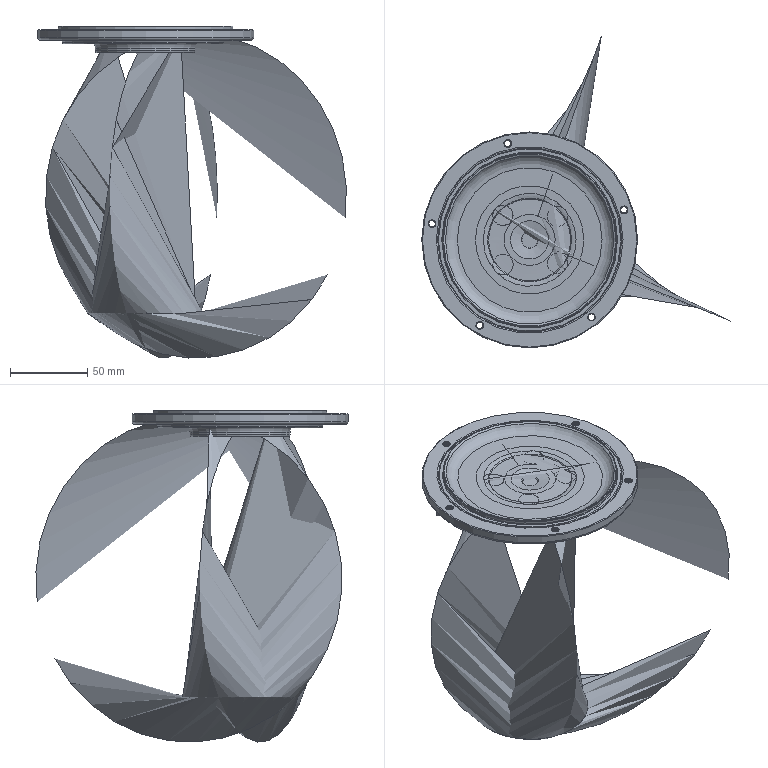CAM job | NX | 3-axis milling, drilling
Tools:
number,name,description,diameter,corner_radius,flute_length,length,flutes
1,D63,Milling Tool-5 Parameters,63.0,0.0,50.0,75.0,2
10,D10,Milling Tool-5 Parameters,10.0,0.0,50.0,75.0,2
11,D10JING,Milling Tool-5 Parameters,10.0,0.0,50.0,75.0,2
6,D6,Milling Tool-5 Parameters,6.0,0.0,50.0,75.0,2
5,D6R0.5,Milling Tool-5 Parameters,6.0,0.5,50.0,75.0,2
2,R0.5,Milling Tool-5 Parameters,1.0,0.5,50.0,75.0,2
7,D6A45,Milling Tool-5 Parameters,6.0,0.0,50.0,75.0,2
3,D3,Milling Tool-5 Parameters,3.0,0.0,50.0,75.0,2
14,4.2ZT,Drilling Tool,4.2,0.0,35.0,50.0,2
16,6.6ZT,Drilling Tool,6.6,0.0,35.0,50.0,2
8,R1.5,Milling Tool-5 Parameters,3.0,1.5,30.0,30.0,4
Operations:
program,operation,operation_type,tool,method,geometry_group,spindle_rpm,surface_speed,feed_per_tooth,feed_cut,feed_plunge,cut_length_mm,path_length_mm,cut_time_min,machine_time_min
1,FLOOR_WALL,VolumeBased25DMillingOperation,D63,METHOD,A,6500.0,1286.0,0.0962,1250.0,100.0,987.547,1041.547,0.79,0.7954
1,ADAPTIVE_MILLING,CavityMilling,D10,METHOD,A,9500.0,298.0,0.1579,3000.0,1000.0,12242.266,12331.08,4.083,4.092
1,CAVITY_MILL,CavityMilling,D10,METHOD,A,9500.0,298.0,0.1579,3000.0,1000.0,13987.132,15102.325,5.036,5.148
1,FLOOR_WALL_1,VolumeBased25DMillingOperation,D10JING,METHOD,A,9500.0,298.0,0.0658,1250.0,100.0,1641.55,1704.25,1.313,1.319
1,ZLEVEL_PROFILE_1,ZLevelMilling,D10JING,METHOD,A,9500.0,298.0,0.0658,1250.0,100.0,478.967,570.782,0.3832,0.3924
1,HOLE_MILLING,CylinderMilling,D6,METHOD,A,9500.0,179.0,0.1053,2000.0,100.0,162.988,239.015,0.0815,0.0891
1,FIXED_CONTOUR,SurfaceContour,D6R0.5,METHOD,A,9500.0,179.0,0.1842,3500.0,1000.0,90276.733,90348.728,25.801,25.808
1,ZLEVEL_PROFILE,ZLevelMilling,D6R0.5,METHOD,A,9500.0,179.0,0.1842,3500.0,1000.0,9728.054,9788.404,2.794,2.8
1,FIXED_CONTOUR_COPY,SurfaceContour,R0.5,METHOD,A,9500.0,179.0,0.1842,3500.0,1000.0,11634.403,11692.003,3.327,3.332
1,PLANAR_MILL,PlanarMilling,D6A45,METHOD,A,9500.0,179.0,0.0789,1500.0,100.0,452.006,516.706,0.3013,0.3078
2,FLOOR_WALL_COPY,VolumeBased25DMillingOperation,D63,METHOD,B,6500.0,1286.0,0.0962,1250.0,100.0,2830.641,3215.735,2.264,2.303
2,CAVITY_MILL_COPY,CavityMilling,D10,METHOD,B,9500.0,298.0,0.1579,3000.0,750.0,28269.25,29278.125,9.95,10.051
2,FLOOR_WALL_1_COPY,VolumeBased25DMillingOperation,D10JING,METHOD,B,9500.0,298.0,0.0658,1250.0,100.0,1599.832,1673.947,1.28,1.287
2,FLOOR_WALL_1_COPY_COPY,VolumeBased25DMillingOperation,D10JING,METHOD,B,9500.0,298.0,0.0658,1250.0,100.0,598.138,663.538,0.4785,0.4851
2,CAVITY_MILL_COPY_COPY,CavityMilling,D6,METHOD,B,9500.0,179.0,0.1053,2000.0,1000.0,1351.467,1851.156,0.7828,0.8328
2,CAVITY_MILL_COPY_COPY_COPY,CavityMilling,D3,METHOD,B,9500.0,89.0,0.0711,1350.0,1000.0,404.339,735.835,0.3226,0.3558
2,DRILLING,Operation,D6A45,METHOD,B,5000.0,94.0,0.025,250.0,0.0,28.0,433.346,0.112,0.1525
2,DRILLING_COPY,Operation,D6A45,METHOD,B,5000.0,94.0,0.025,250.0,0.0,22.4,218.986,0.0896,0.1093
2,DRILLING_COPY_1,Operation,4.2ZT,METHOD,B,2000.0,26.0,0.0625,250.0,0.0,61.309,499.964,0.2452,0.2891
2,DRILLING_COPY_COPY,Operation,6.6ZT,METHOD,B,2000.0,41.0,0.0625,250.0,0.0,59.931,294.049,0.2397,0.2631
2,PLANAR_MILL_COPY,PlanarMilling,D6A45,METHOD,B,9500.0,179.0,0.0789,1500.0,100.0,85.363,452.323,0.0569,0.0936
2,ZLEVEL_PROFILE_COPY,ZLevelMilling,D6R0.5,METHOD,B,9500.0,179.0,0.1842,3500.0,1000.0,3101.647,3173.346,0.9003,0.9074
2,FIXED_CONTOUR_COPY_1_COPY_COPY,SurfaceContour,D6R0.5,METHOD,B,9500.0,179.0,0.1842,3500.0,1000.0,70122.253,70181.666,20.038,20.044
2,ZLEVEL_PROFILE_COPY_1,ZLevelMilling,D6R0.5,METHOD,B,9500.0,179.0,0.1842,3500.0,1000.0,17246.31,17322.924,4.941,4.949
2,ZLEVEL_PROFILE_COPY_1_COPY,ZLevelMilling,D6R0.5,METHOD,B,9500.0,179.0,0.1842,3500.0,1000.0,7565.946,7627.646,2.175,2.182
2,ZLEVEL_PROFILE_COPY_1_COPY_COPY,ZLevelMilling,D6R0.5,METHOD,B,9500.0,179.0,0.1842,3500.0,1000.0,780.854,852.914,0.2378,0.245
2,FIXED_CONTOUR_COPY_1,SurfaceContour,R1.5,METHOD,B,9500.0,179.0,0.1842,3500.0,1000.0,26540.031,26603.631,7.586,7.593